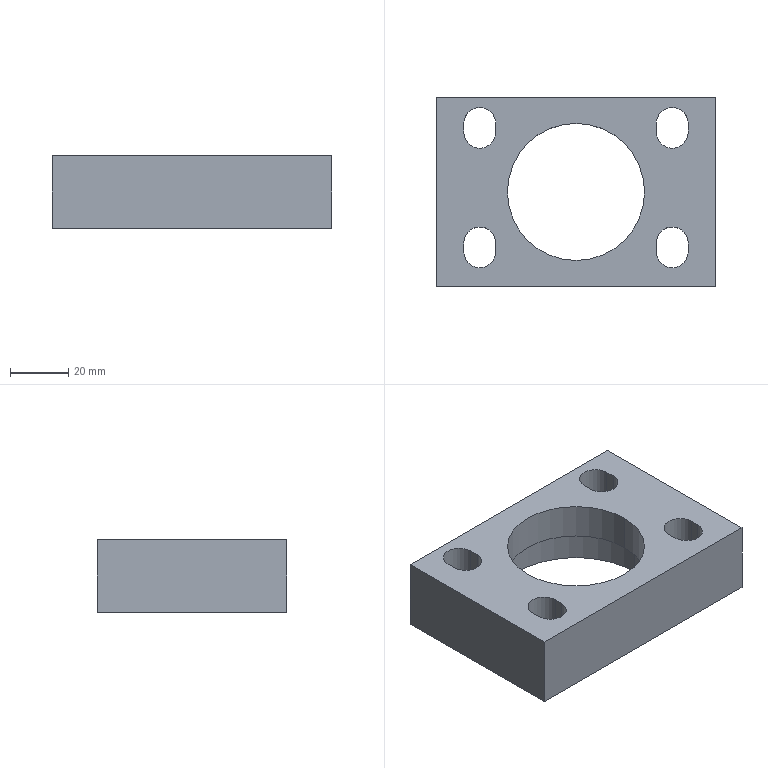Part | STEP file | GA DAU NOI VAO DAU BUA | 1 solid | 27 faces | box 96 x 65 x 25 mm | volume 89450 mm3 | plane 15 | cylinder 12 | commonest cylinder face diameters 11 x8 47 x2 57 x2